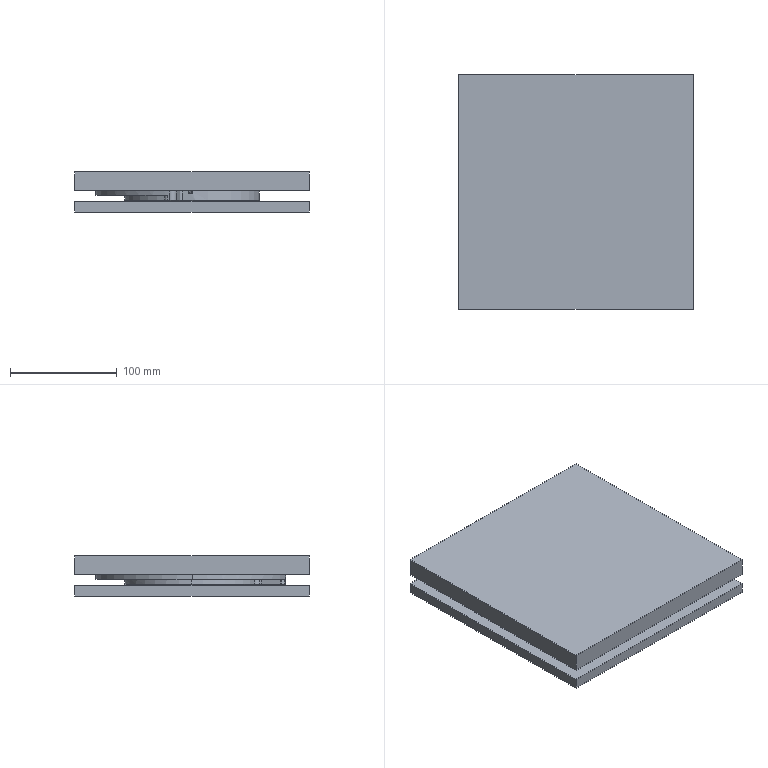NC program | NX | posted with a generic post | part box 220 x 220 x 37.5 mm
Lines 76 to 952 of 13716:
(ADAPTIVE_MILLING , TOOL : D10)
N120 T03 M6
N122 G54
N124 G17 G0 G90 X86.367 Y-45.277 S8000 M3
N126 G43 Z30. H3
N128 Z-14.
N130 G94 G1 Z-17. F1000.
N132 X84.574 Y-44.181 F3500.
N134 G3 X83.996 Y-44.309 R0.517
N136 X80.048 Y-49.358 R33.84
N138 G2 X66.319 Y-66.497 R105.778
N140 X-92.415 Y16.802 R93.928
N142 X-92.829 Y20.13 R11.157
N144 G3 X-93.451 Y20.622 R0.524
N146 G1 X-95.297 Y20.256
N148 G3 X-95.297 Y19.277 R0.523
N150 G1 Z-14.
N152 G0 Z30.
N154 X84.745 Y-47.205
N156 Z-14.
N158 G1 Z-17. F1000.
N160 G3 X85.138 Y-46.276 R0.505 F3500.
N162 G1 X83.355 Y-45.432
N164 G3 X82.875 Y-45.546 R0.516
N166 X78.753 Y-49.761 R17.096
N168 G2 X70.173 Y-60.818 R172.579
N170 X-91.735 Y14.531 R92.876
N172 G1 X-91.721 Y14.655
N174 X-91.709 Y14.779
N176 X-91.702 Y14.904
N178 X-91.718 Y15.028
N180 X-91.723 Y15.053
N182 G2 X-92.422 Y16.833 R12.053
N184 G3 X-93.208 Y17.162 R0.523
N186 G1 X-94.72 Y16.21
N188 G3 X-94.552 Y15.325 R0.523
N190 G1 Z-14.
N192 G0 Z30.
N194 X83.381 Y-48.311
N196 Z-14.
N198 G1 Z-17. F1000.
N200 G3 X83.835 Y-47.418 R0.505 F3500.
N202 G1 X82.268 Y-46.36
N204 G3 X81.746 Y-46.416 R0.514
N206 G2 X80.496 Y-47.163 R8.174
N208 G3 X77.305 Y-50.313 R15.899
N210 G2 X69.954 Y-59.478 R395.084
N212 X-90.974 Y12.49 R91.836
N214 G3 X-90.988 Y13.871 R3.68
N216 G2 X-91.754 Y15.127 R8.922
N218 G3 X-92.604 Y15.292 R0.523
N220 G1 X-93.829 Y14.054
N222 G3 X-93.578 Y13.261 R0.524
N224 G1 Z-14.
N226 G0 Z30.
N228 X82.131 Y-49.111
N230 Z-14.
N232 G1 Z-17. F1000.
N234 G3 X82.626 Y-48.25 R0.505 F3500.
N236 G1 X81.197 Y-47.049
N238 G3 X80.71 Y-47.033 R0.516
N240 X78.354 Y-48.358 R13.575
N242 X74.556 Y-52.323 R27.605
N244 G2 X65.409 Y-62.915 R164.628
N246 X-90.181 Y10.267 R90.765
N248 G3 X-90.157 Y12.759 R9.982
N250 X-90.653 Y13.361 R2.719
N252 G1 X-90.996 Y13.883
N254 G3 X-91.709 Y14.019 R0.507
N256 G1 X-93.073 Y13.05
N258 G3 X-92.887 Y12.216 R0.506
N260 G1 Z-14.
N262 G0 Z30.
N264 X80.927 Y-49.729
N266 Z-14.
N268 G1 Z-17. F1000.
N270 G3 X81.459 Y-48.902 R0.505 F3500.
N272 G1 X80.19 Y-47.603
N274 G3 X79.742 Y-47.523 R0.518
N276 X75.889 Y-49.733 R8.088
N278 X70.939 Y-55.194 R66.815
N280 G2 X58.211 Y-68.242 R108.748
N282 X-89.332 Y8.128 R89.703
N284 G3 X-89.304 Y11.744 R15.899
N286 G1 X-89.33 Y11.866
N288 X-89.376 Y11.983
N290 X-89.432 Y12.077
N292 X-90.295 Y12.98
N294 G3 X-90.994 Y13.011 R0.508
N296 G1 X-92.213 Y11.927
N298 G3 X-91.988 Y11.136 R0.507
N300 G1 Z-14.
N302 G0 Z30.
N304 X79.741 Y-50.13
N306 Z-14.
N308 G1 Z-17. F1000.
N310 G3 X80.32 Y-49.359 R0.505 F3500.
N312 G1 X79.288 Y-47.939
N314 G3 X78.784 Y-47.81 R0.514
N316 X76.695 Y-48.509 R11.339
N318 X72.855 Y-51.682 R16.957
N320 X65.561 Y-59.747 R993.743
N322 G2 X9.214 Y-88.161 R89.35
N324 X-88.406 Y6.532 R88.653
N326 G3 X-88.422 Y10.773 R20.785
N328 X-88.714 Y11.536 R1.595
N330 G1 X-89.35 Y11.998
N332 X-89.389 Y12.031
N334 X-89.475 Y12.122
N336 G3 X-90.244 Y12.076 R0.507
N338 G1 X-91.21 Y10.779
N340 G3 X-90.931 Y10.072 R0.507
N342 G1 Z-14.
N344 G0 Z30.
N346 X78.751 Y-50.429
N348 Z-14.
N350 G1 Z-17. F1000.
N352 G3 X79.348 Y-49.685 R0.505 F3500.
N354 G1 X78.418 Y-48.214
N356 G3 X77.983 Y-48.045 R0.517
N358 X74.203 Y-49.513 R6.431
N360 X69.408 Y-54.07 R36.849
N362 G2 X59.034 Y-64.722 R153.931
N364 X-87.451 Y5.032 R87.61
N366 G3 X-87.519 Y9.898 R25.802
N368 X-87.906 Y10.951 R2.017
N370 G1 X-88.715 Y11.537
N372 G3 X-89.438 Y11.399 R0.507
N374 G1 X-90.286 Y10.052
N376 G3 X-89.992 Y9.378 R0.507
N378 G1 Z-14.
N380 G0 Z30.
N382 X77.512 Y-50.61
N384 Z-14.
N386 G1 Z-17. F1000.
N388 G3 X78.146 Y-49.934 R0.506 F3500.
N390 G1 X77.47 Y-48.386
N392 G3 X76.989 Y-48.155 R0.513
N394 X72.903 Y-49.694 R7.007
N396 X67.694 Y-54.54 R40.76
N398 G2 X57.321 Y-64.841 R147.601
N400 X-86.479 Y2.946 R86.546
N402 G3 X-86.557 Y8.814 R40.487
N404 X-87.061 Y10.476 R4.512
N406 X-87.906 Y10.951 R3.058
N408 X-88.509 Y10.885 R0.51
N410 G1 X-89.688 Y9.772
N412 G3 X-89.456 Y8.992 R0.507
N414 G1 Z-14.
N416 G0 Z30.
N418 X76.508 Y-50.724
N420 Z-14.
N422 G1 Z-17. F1000.
N424 G3 X77.155 Y-50.078 R0.506 F3500.
N426 G1 X76.584 Y-48.502
N428 G3 X76.178 Y-48.244 R0.516
N430 X72.949 Y-48.977 R5.032
N432 X68.167 Y-52.774 R23.029
N434 G2 X60.321 Y-60.66 R868.911
N436 X17.03 Y-83.76 R86.865
N438 X-85.46 Y1.604 R85.487
N440 G3 X-85.609 Y7.973 R49.447
N442 X-86.267 Y10.105 R5.323
N444 X-87.303 Y10.657 R4.211
N446 X-87.985 Y10.401 R0.507
N448 G1 X-88.599 Y8.951
N450 G3 X-88.28 Y8.355 R0.508
N452 G1 Z-14.
N454 G0 Z30.
N456 X75.748 Y-50.717
N458 Z-14.
N460 G1 Z-17. F1000.
N462 G3 X76.408 Y-50.115 R0.506 F3500.
N464 G1 X75.982 Y-48.502
N466 G3 X75.555 Y-48.2 R0.514
N468 X71.611 Y-49.072 R5.827
N470 X66.358 Y-53.283 R27.528
N472 G2 X57.105 Y-62.233 R285.389
N474 X-22.068 Y-81.479 R84.739
N476 X-84.42 Y1.361 R84.539
N478 G3 X-84.713 Y7.598 R42.846
N480 X-85.578 Y9.91 R4.764
N482 X-86.252 Y10.155 R2.421
N484 G1 X-86.478 Y10.262
N486 G3 X-87.096 Y10.115 R0.509
N488 G1 X-88.072 Y8.837
N490 G3 X-87.797 Y8.126 R0.507
N492 G1 Z-14.
N494 G0 Z30.
N496 X74.669 Y-50.642
N498 Z-14.
N500 G1 Z-17. F1000.
N502 G3 X75.342 Y-50.103 R0.506 F3500.
N504 G1 X75.129 Y-48.493
N506 G3 X74.682 Y-48.138 R0.512
N508 X73.338 Y-48.022 R8.372
N510 X69.453 Y-49.64 R8.896
N512 X64.035 Y-54.253 R41.121
N514 G2 X53.368 Y-64.067 R172.763
N516 X-83.361 Y-0.32 R83.394
N518 G3 X-83.693 Y6.543 R61.748
N520 X-84.718 Y9.593 R6.709
N522 G1 X-84.801 Y9.686
N524 X-84.902 Y9.76
N526 X-84.99 Y9.807
N528 X-85.834 Y10.036
N530 G3 X-86.45 Y9.694 R0.508
N532 G1 X-86.896 Y8.181
N534 G3 X-86.567 Y7.645 R0.509
N536 G1 Z-14.
N538 G0 Z30.
N540 X74.105 Y-50.594
N542 Z-14.
N544 G1 Z-17. F1000.
N546 G3 X74.778 Y-50.056 R0.506 F3500.
N548 G1 X74.564 Y-48.419
N550 G3 X74.207 Y-48.077 R0.515
N552 X70.675 Y-48.288 R4.771
N554 X65.767 Y-51.471 R18.618
N556 X58.324 Y-58.334 R265.551
N558 G2 X38.9 Y-72.524 R91.967
N560 X-82.285 Y-1.651 R82.313
N562 G3 X-82.729 Y5.957 R72.331
N564 X-83.817 Y9.254 R8.109
N566 X-84.47 Y9.666 R0.828
N568 G1 X-85.073 Y9.83
N570 G3 X-85.699 Y9.449 R0.507
N572 G1 X-86.026 Y7.91
N574 G3 X-85.694 Y7.409 R0.51
N576 G1 Z-14.
N578 G0 Z30.
N580 X73.24 Y-50.406
N582 Z-14.
N584 G1 Z-17. F1000.
N586 G3 X73.918 Y-49.912 R0.507 F3500.
N588 G1 X73.851 Y-48.28
N590 G3 X73.481 Y-47.89 R0.514
N592 X69.671 Y-48.101 R5.133
N594 X64.343 Y-51.553 R20.596
N596 X56.082 Y-59.004 R405.756
N598 G2 X36.408 Y-72.62 R89.446
N600 X-81.179 Y-3.094 R81.248
N602 G3 X-81.711 Y5.135 R96.899
N604 X-82.901 Y8.924 R9.743
N606 X-83.488 Y9.492 R1.449
N608 G1 X-84.35 Y9.644
N610 G3 X-84.935 Y9.237 R0.507
N612 G1 X-85.21 Y7.685
N614 G3 X-84.878 Y7.198 R0.51
N616 G1 Z-14.
N618 G0 Z30.
N620 X72.201 Y-50.141
N622 Z-14.
N624 G1 Z-17. F1000.
N626 G3 X72.879 Y-49.685 R0.507 F3500.
N628 G1 X72.932 Y-48.078
N630 G3 X72.6 Y-47.663 R0.513
N632 X69.866 Y-47.501 R3.861
N634 X64.896 Y-50.062 R14.817
N636 X58.048 Y-55.894 R92.054
N638 G2 X45.619 Y-65.951 R118.839
N640 X-80.105 Y-3.568 R80.212
N642 G3 X-80.756 Y4.778 R92.475
N644 X-82.088 Y8.78 R10.206
N646 X-82.682 Y9.35 R1.491
N648 G1 X-83.544 Y9.502
N650 G3 X-84.133 Y9.066 R0.507
N652 G1 X-84.318 Y7.492
N654 G3 X-83.987 Y7.041 R0.512
N656 G1 Z-14.
N658 G0 Z30.
N660 X71.367 Y-49.848
N662 Z-14.
N664 G1 Z-17. F1000.
N666 G3 X72.007 Y-49.568 R0.508 F3500.
N668 G1 X72.606 Y-48.112
N670 G3 X72.326 Y-47.541 R0.509
N672 X68.936 Y-47.222 R4.324
N674 X63.74 Y-49.891 R15.977
N676 X56.554 Y-55.906 R102.667
N678 G2 X43.355 Y-66.192 R112.499
N680 X-79.021 Y-4.133 R79.167
N682 G3 X-79.796 Y4.454 R91.307
N684 X-81.27 Y8.67 R10.869
N686 X-81.843 Y9.202 R1.569
N688 G1 X-82.705 Y9.354
N690 G3 X-83.26 Y9.051 R0.512
N692 G1 X-83.881 Y7.562
N694 G3 X-83.563 Y6.966 R0.511
N696 G1 Z-14.
N698 G0 Z30.
N700 X71.078 Y-49.715
N702 Z-14.
N704 G1 Z-17. F1000.
N706 G3 X71.76 Y-49.294 R0.512 F3500.
N708 G1 X71.941 Y-47.668
N710 G3 X71.645 Y-47.226 R0.519
N712 X68.131 Y-46.887 R4.547
N714 X62.793 Y-49.552 R16.49
N716 X55.348 Y-55.646 R104.608
N718 G2 X40.868 Y-66.511 R108.174
N720 X-77.901 Y-5.089 R78.108
N722 G3 X-78.721 Y3.494 R117.25
N724 X-80.218 Y8.233 R13.248
N726 X-80.991 Y9.051 R1.926
N728 G1 X-81.852 Y9.203
N730 G3 X-82.413 Y8.883 R0.51
N732 G1 X-82.97 Y7.381
N734 G3 X-82.649 Y6.805 R0.509
N736 G1 Z-14.
N738 G0 Z30.
N740 X70.294 Y-49.355
N742 Z-14.
N744 G1 Z-17. F1000.
N746 G3 X70.966 Y-48.973 R0.509 F3500.
N748 G1 X71.258 Y-47.382
N750 G3 X70.964 Y-46.912 R0.514
N752 X67.886 Y-46.418 R4.123
N754 X62.533 Y-48.742 R14.766
N756 X55.061 Y-54.599 R79.752
N758 G2 X41.84 Y-64.655 R119.816
N760 X-76.751 Y-6.254 R77.047
N762 G3 X-77.721 Y3.068 R142.072
N764 X-79.247 Y7.933 R14.664
N766 X-80.113 Y8.897 R2.203
N768 G1 X-81.098 Y9.07
N770 G3 X-81.665 Y8.732 R0.509
N772 G1 X-82.161 Y7.211
N774 G3 X-81.836 Y6.662 R0.509
N776 G1 Z-14.
N778 G0 Z30.
N780 X69.384 Y-48.891
N782 Z-14.
N784 G1 Z-17. F1000.
N786 G3 X69.992 Y-48.674 R0.509 F3500.
N788 G1 X70.791 Y-47.316
N790 G3 X70.574 Y-46.693 R0.509
N792 X67.112 Y-46.033 R4.424
N794 X61.52 Y-48.429 R15.36
N796 X54.186 Y-54.057 R77.463
N798 G2 X41.309 Y-63.743 R126.175
N800 X-75.59 Y-7.267 R75.998
N802 G3 X-76.698 Y2.544 R174.092
N804 X-78.341 Y7.762 R15.754
N806 X-79.22 Y8.739 R2.223
N808 G1 X-80.205 Y8.913
N810 G3 X-80.775 Y8.565 R0.509
N812 G1 X-81.24 Y7.039
N814 G3 X-80.914 Y6.499 R0.509
N816 G1 Z-14.
N818 G0 Z30.
N820 X69.11 Y-48.733
N822 Z-14.
N824 G1 Z-17. F1000.
N826 G3 X69.78 Y-48.381 R0.512 F3500.
N828 G1 X70.177 Y-46.804
N830 G3 X69.924 Y-46.318 R0.518
N832 X66.343 Y-45.629 R4.585
N834 X60.618 Y-48.031 R15.844
N836 X53.809 Y-53.111 R72.764
N838 G2 X41.843 Y-62.143 R146.46
N840 X-32.178 Y-67.574 R75.192
N842 X-74.499 Y-7.548 R75.061
N844 G3 X-75.726 Y2.374 R170.304
N846 X-77.416 Y7.58 R16.3
N848 X-78.323 Y8.581 R2.263
N850 G1 X-79.308 Y8.755
N852 G3 X-79.88 Y8.4 R0.509
N854 G1 X-80.324 Y6.872
N856 G3 X-79.997 Y6.338 R0.509
N858 G1 Z-14.
N860 G0 Z30.
N862 X68.393 Y-48.319
N864 Z-14.
N866 G1 Z-17. F1000.
N868 G3 X69.052 Y-47.993 R0.509 F3500.
N870 G1 X69.524 Y-46.448
N872 G3 X69.275 Y-45.943 R0.514
N874 X65.578 Y-45.213 R4.742
N876 X59.932 Y-47.49 R15.988
N878 X53.059 Y-52.481 R68.743
N880 G2 X41.129 Y-61.355 R153.462
N882 X-20.52 Y-70.866 R74.359
N884 X-73.248 Y-9.08 R73.915
N886 G3 X-74.571 Y1.21 R390.61
N888 X-76.24 Y6.95 R20.325
N890 X-77.265 Y8.352 R4.627
N892 X-78.391 Y8.593 R5.382
N894 X-78.964 Y8.236 R0.508
N896 G1 X-79.398 Y6.706
N898 G3 X-79.07 Y6.174 R0.509
N900 G1 Z-14.
N902 G0 Z30.
N904 X67.578 Y-47.849
N906 Z-14.
N908 G1 Z-17. F1000.
N910 G3 X68.229 Y-47.545 R0.507 F3500.
N912 G1 X68.761 Y-46.037
N914 G3 X68.517 Y-45.505 R0.51
N916 X64.939 Y-44.767 R4.751
N918 X59.146 Y-47.003 R15.989
N920 X51.231 Y-52.685 R75.994
N922 G2 X38.947 Y-61.495 R138.42
N924 X-26.793 Y-67.595 R73.2
N926 X-72.139 Y-9.381 R72.911
N928 G3 X-73.555 Y0.896 R384.559
N930 X-75.348 Y6.859 R20.943
N932 X-76.411 Y8.226 R3.68
N934 G1 X-76.485 Y8.257
N936 X-77.47 Y8.431
N938 G3 X-78.043 Y8.073 R0.508
N940 G1 X-78.477 Y6.543
N942 G3 X-78.15 Y6.012 R0.509
N944 G1 Z-14.
N946 G0 Z30.
N948 X66.767 Y-47.381
N950 Z-14.
N952 G1 Z-17. F1000.
N954 G3 X67.41 Y-47.095 R0.508 F3500.
N956 G1 X67.999 Y-45.617
N958 G3 X67.759 Y-45.068 R0.51
N960 X64.053 Y-44.348 R4.931
N962 X57.928 Y-46.76 R17.069
N964 X49.689 Y-52.636 R89.664
N966 G2 X37.389 Y-61.206 R128.95
N968 X-32.584 Y-63.804 R72.032
N970 X-71.044 Y-9.564 R71.967
N972 G3 X-72.606 Y0.944 R299.425
N974 X-74.444 Y6.763 R20.566
N976 X-75.43 Y8.038 R4.3
N978 X-76.539 Y8.266 R11.317
N980 X-77.111 Y7.909 R0.508
N982 G1 X-77.545 Y6.379
N984 G3 X-77.218 Y5.848 R0.509
N986 G1 Z-14.
N988 G0 Z30.
N990 X66.101 Y-46.996
N992 Z-14.
N994 G1 Z-17. F1000.
N996 G3 X66.742 Y-46.717 R0.508 F3500.
N998 G1 X67.348 Y-45.248
N1000 G3 X67.11 Y-44.693 R0.51
N1002 X63.294 Y-43.9 R5.074
N1004 X57.144 Y-46.251 R17.239
N1006 X49.445 Y-51.59 R84.212
N1008 G2 X37.556 Y-59.88 R144.347
N1010 X-11.773 Y-69.586 R71.533
N1012 X-69.773 Y-10.869 R70.78
N1014 G3 X-71.458 Y0.001 R801.947
N1016 X-73.295 Y6.215 R24.669
N1018 X-74.436 Y7.842 R5.577
N1020 X-75.586 Y8.098 R4.111
N1022 X-76.161 Y7.732 R0.508
N1024 G1 X-76.566 Y6.198
N1026 G3 X-76.238 Y5.675 R0.51
N1028 G1 Z-14.
N1030 G0 Z30.
N1032 X65.325 Y-46.548
N1034 Z-14.
N1036 G1 Z-17. F1000.
N1038 G3 X65.963 Y-46.275 R0.508 F3500.
N1040 G1 X66.589 Y-44.816
N1042 G3 X66.352 Y-44.255 R0.51
N1044 X62.538 Y-43.443 R5.132
N1046 X56.365 Y-45.736 R17.413
N1048 X48.11 Y-51.368 R85.254
N1050 G2 X36.226 Y-59.443 R137.297
N1052 X-19.674 Y-66.662 R70.27
N1054 X-68.706 Y-10.821 R69.795
N1056 G3 X-70.542 Y0.278 R462.541
N1058 X-72.487 Y6.326 R22.468
N1060 X-73.542 Y7.705 R4.592
N1062 X-74.65 Y7.933 R11.921
N1064 X-75.236 Y7.513 R0.507
N1066 G1 X-75.472 Y5.946
N1068 G3 X-75.142 Y5.481 R0.512
N1070 G1 Z-14.
N1072 G0 Z30.
N1074 X64.56 Y-46.107
N1076 Z-14.
N1078 G1 Z-17. F1000.
N1080 G3 X65.198 Y-45.836 R0.508 F3500.
N1082 G1 X65.831 Y-44.381
N1084 G3 X65.594 Y-43.818 R0.51
N1086 X61.659 Y-42.996 R5.246
N1088 X55.587 Y-45.21 R17.735
N1090 X47.176 Y-50.835 R86.711
N1092 G2 X34.897 Y-58.993 R133.657
N1094 X-18.089 Y-66. R69.271
N1096 X-67.485 Y-11.64 R68.736
N1098 G3 X-69.423 Y-0.432 R902.29
N1100 X-71.436 Y5.989 R25.143
N1102 X-72.638 Y7.562 R4.16
N1104 G1 X-72.707 Y7.591
N1106 X-73.691 Y7.764
N1108 G3 X-74.276 Y7.358 R0.507
N1110 G1 X-74.552 Y5.806
N1112 G3 X-74.223 Y5.319 R0.51
N1114 G1 Z-14.
N1116 G0 Z30.
N1118 X63.803 Y-45.669
N1120 Z-14.
N1122 G1 Z-17. F1000.
N1124 G3 X64.44 Y-45.399 R0.508 F3500.
N1126 G1 X65.073 Y-43.943
N1128 G3 X64.836 Y-43.38 R0.51
N1130 X60.906 Y-42.526 R5.297
N1132 X54.485 Y-44.862 R18.154
N1134 X45.736 Y-50.658 R95.431
N1136 X42.203 Y-53.51 R36.5
N1138 G1 X38.136 Y-56.48
N1140 X38.119 Y-56.492
N1142 X33.843 Y-59.152
N1144 X33.825 Y-59.163
N1146 X29.364 Y-61.499
N1148 X29.345 Y-61.508
N1150 X24.724 Y-63.507
N1152 X24.704 Y-63.514
N1154 X19.947 Y-65.165
N1156 X19.927 Y-65.171
N1158 X15.06 Y-66.465
N1160 X15.04 Y-66.469
N1162 X10.091 Y-67.398
N1164 X10.07 Y-67.402
N1166 X5.065 Y-67.961
N1168 X5.045 Y-67.963
N1170 X0.002 Y-68.15
N1172 X-5.134 Y-67.956
N1174 X-5.155 Y-67.954
N1176 X-10.251 Y-67.374
N1178 X-10.272 Y-67.371
N1180 X-15.31 Y-66.408
N1182 X-15.33 Y-66.403
N1184 X-20.281 Y-65.062
N1186 X-20.301 Y-65.056
N1188 X-25.136 Y-63.345
N1190 X-25.156 Y-63.337
N1192 X-29.848 Y-61.265
N1194 X-29.867 Y-61.256
N1196 X-34.39 Y-58.836
N1198 X-34.408 Y-58.826
N1200 X-38.735 Y-56.071
N1202 X-38.752 Y-56.059
N1204 X-42.858 Y-52.986
N1206 X-42.875 Y-52.973
N1208 X-46.737 Y-49.598
N1210 X-46.753 Y-49.584
N1212 X-50.35 Y-45.927
N1214 X-50.364 Y-45.911
N1216 X-53.674 Y-41.994
N1218 X-53.687 Y-41.977
N1220 X-56.692 Y-37.82
N1222 X-56.704 Y-37.803
N1224 X-59.386 Y-33.431
N1226 X-59.397 Y-33.413
N1228 X-61.741 Y-28.851
N1230 X-61.75 Y-28.832
N1232 X-63.744 Y-24.106
N1234 X-63.751 Y-24.086
N1236 X-65.382 Y-19.223
N1238 X-65.388 Y-19.203
N1240 X-66.647 Y-14.231
N1242 X-66.652 Y-14.21
N1244 X-67.532 Y-9.157
N1246 X-67.534 Y-9.136
N1248 G3 X-68.392 Y-1.159 R141.378
N1250 X-70.446 Y5.767 R24.619
N1252 X-71.622 Y7.365 R5.084
N1254 X-72.734 Y7.595 R8.834
N1256 X-73.363 Y6.923 R0.551
N1258 G1 X-72.651 Y5.054 Z-16.9
N1260 X-70.616 Y-0.252
N1262 X-69.9 Y-2.119 Z-17.
N1264 X-69.056 Y-4.3
N1266 G3 X-68.032 Y-4.01 R0.55
N1268 X-68.201 Y1.11 R67.977
N1270 X-70.205 Y6.706 R12.59
N1272 X-70.809 Y7.256 R1.69
N1274 G1 X-71.794 Y7.43
N1276 G3 X-72.384 Y6.649 R0.551
N1278 G1 X-69.123 Y-0.088
N1280 G3 X-68.122 Y0.239 R0.55
N1282 G2 X-68.09 Y2.759 R104.092
N1284 G3 X-69.652 Y6.901 R7.194
N1286 G1 X-69.741 Y6.989
N1288 X-69.846 Y7.058
N1290 X-69.961 Y7.107
N1292 X-70.823 Y7.259
N1294 G3 X-71.407 Y6.464 R0.551
N1296 G1 X-69.069 Y1.961
N1298 G3 X-68.079 Y2.259 R0.551
N1300 X-68.086 Y4.876 R10.598
N1302 X-69.052 Y6.873 R3.968
N1304 X-70.001 Y7.114 R2.516
N1306 X-70.571 Y6.294 R0.551
N1308 G1 X-68.964 Y3.562
N1310 G3 X-67.991 Y3.882 R0.551
N1312 X-68.08 Y5.989 R5.552
N1314 X-68.751 Y6.893 R1.35
N1316 G1 X-69.366 Y7.002
N1318 G3 X-69.914 Y6.148 R0.551
N1320 G1 X-68.874 Y4.653
N1322 G3 X-67.93 Y5.005 R0.551
N1324 X-68.051 Y6.48 R2.883
N1326 X-68.816 Y6.905 R0.857
N1328 X-69.337 Y6.015 R0.551
N1330 G1 X-68.803 Y5.373
N1332 G3 X-67.889 Y5.754 R0.551
N1334 X-67.994 Y6.595 R1.279
N1336 X-68.499 Y6.849 R0.878
N1338 X-68.91 Y6.772 R0.63
N1340 G1 X-70.702 Y5.686
N1342 G3 X-70.531 Y4.669 R0.597
N1344 G1 Z-14.
N1346 G0 Z30.
N1348 X63.045 Y-45.232
N1350 Z-14.
N1352 G1 Z-17. F1000.
N1354 G3 X63.684 Y-44.961 R0.508 F3500.
N1356 G1 X64.315 Y-43.505
N1358 G3 X64.079 Y-42.943 R0.51
N1360 X60.03 Y-42.063 R5.422
N1362 X53.709 Y-44.321 R18.66
N1364 X49.349 Y-46.979 R71.69
N1366 G1 X46.069 Y-50.219
N1368 X46.054 Y-50.234
N1370 X44.626 Y-51.449
N1372 G3 X45.228 Y-52.36 R0.55
N1374 G1 X47.922 Y-51.017
N1376 X49.712 Y-50.125 Z-16.9
N1378 X61.396 Y-44.302
N1380 X63.186 Y-43.409 Z-17.
N1382 G3 X63.213 Y-42.443 R0.551
N1384 X59.28 Y-41.584 R5.413
N1386 X53.047 Y-43.719 R18.361
N1388 G1 X52.825 Y-43.836
N1390 X52.605 Y-43.954
N1392 X52.166 Y-44.193
N1394 X51.839 Y-44.376
N1396 X51.621 Y-44.5
N1398 X51.514 Y-44.564
N1400 X51.472 Y-44.595
N1402 G2 X49.296 Y-47.032 R68.293
N1404 G3 X49.885 Y-47.935 R0.55
N1406 G1 X51.047 Y-47.475
N1408 X52.907 Y-46.74 Z-16.9
N1410 X60.456 Y-43.754
N1412 X62.316 Y-43.019 Z-17.
N1414 G3 X62.455 Y-42.005 R0.554
N1416 X58.406 Y-41.112 R5.513
N1418 X52.993 Y-42.85 R16.487
N1420 G1 X52.976 Y-42.871
N1422 X51.415 Y-44.66
N1424 G3 X51.997 Y-45.546 R0.55
N1426 G1 X61.565 Y-42.47
N1428 G3 X61.589 Y-41.505 R0.551
N1430 X57.658 Y-40.619 R5.484
N1432 X53.935 Y-41.613 R11.166
N1434 G1 X53.892 Y-41.65
N1436 X52.989 Y-42.854
N1438 G3 X53.553 Y-43.72 R0.551
N1440 G1 X60.763 Y-42.053
N1442 G3 X60.831 Y-41.068 R0.551
N1444 X56.788 Y-40.136 R5.589
N1446 X54.725 Y-40.607 R7.529
N1448 X53.852 Y-41.703 R6.836
N1450 X54.392 Y-42.574 R0.551
N1452 G1 X59.875 Y-41.562
N1454 G3 X59.965 Y-40.568 R0.551
N1456 X55.319 Y-39.85 R5.283
N1458 X54.548 Y-40.774 R3.656
N1460 X55.068 Y-41.648 R0.551
N1462 G1 X58.992 Y-41.068
N1464 G3 X59.099 Y-40.068 R0.551
N1466 X56.291 Y-39.198 R4.57
N1468 X55.547 Y-39.442 R1.289
N1470 G1 X55.097 Y-40.042
N1472 G3 X55.611 Y-40.917 R0.551
N1474 G1 X58.121 Y-40.569
N1476 G3 X58.233 Y-39.568 R0.551
N1478 X56.389 Y-38.884 R3.466
N1480 X55.807 Y-39.094 R0.897
N1482 G1 X55.507 Y-39.494
N1484 G3 X56.042 Y-40.366 R0.551
N1486 G1 X57.381 Y-40.126
N1488 G3 X57.475 Y-39.13 R0.551
N1490 X56.324 Y-38.707 R2.025
N1492 X55.733 Y-39.193 R0.951
N1494 X56.322 Y-40.052 R0.55
N1496 G1 X56.996 Y-39.857
N1498 G3 X57.042 Y-38.88 R0.551
N1500 X56.094 Y-38.763 R0.805
N1502 G1 X55.958 Y-38.893
N1504 G3 X55.893 Y-39.51 R0.615
N1506 G1 X56.933 Y-41.761
N1508 Z-14.
N1510 G0 Z30.
N1512 X41.169 Y-27.555
N1514 Z3.
N1516 G3 X41.169 Y-27.555 Z2.506 I0.978 J4.392 F1000.
N1518 X41.169 Y-27.555 Z2.013 I0.978 J4.392
N1520 X41.169 Y-27.555 Z1.519 I0.978 J4.392
N1522 X41.169 Y-27.555 Z1.026 I0.978 J4.392
N1524 X41.169 Y-27.555 Z0.532 I0.978 J4.392
N1526 X41.169 Y-27.555 Z0.039 I0.978 J4.392
N1528 X41.169 Y-27.555 Z-0.455 I0.978 J4.392
N1530 X41.169 Y-27.555 Z-0.948 I0.978 J4.392
N1532 X41.169 Y-27.555 Z-1.442 I0.978 J4.392
N1534 X41.169 Y-27.555 Z-1.935 I0.978 J4.392
N1536 X41.169 Y-27.555 Z-2.429 I0.978 J4.392
N1538 X41.169 Y-27.555 Z-2.922 I0.978 J4.392
N1540 X41.169 Y-27.555 Z-3.416 I0.978 J4.392
N1542 X41.169 Y-27.555 Z-3.909 I0.978 J4.392
N1544 X41.169 Y-27.555 Z-4.403 I0.978 J4.392
N1546 X41.169 Y-27.555 Z-4.896 I0.978 J4.392
N1548 X41.169 Y-27.555 Z-5.39 I0.978 J4.392
N1550 X41.169 Y-27.555 Z-5.884 I0.978 J4.392
N1552 X41.169 Y-27.555 Z-6.377 I0.978 J4.392
N1554 X41.169 Y-27.555 Z-6.871 I0.978 J4.392
N1556 X41.169 Y-27.555 Z-7.364 I0.978 J4.392
N1558 X41.169 Y-27.555 Z-7.858 I0.978 J4.392
N1560 X41.169 Y-27.555 Z-8.351 I0.978 J4.392
N1562 X41.169 Y-27.555 Z-8.845 I0.978 J4.392
N1564 X41.169 Y-27.555 Z-9.338 I0.978 J4.392
N1566 X41.169 Y-27.555 Z-9.832 I0.978 J4.392
N1568 X42.148 Y-27.663 Z-9.849 R4.5
N1570 X39.542 Y-26.842 R-4.501 F3500.
N1572 X47.015 Y-22.173 R4.667
N1574 X38.677 Y-26.748 R-4.976
N1576 X47.243 Y-21.2 R5.196
N1578 X38.066 Y-26.845 R-5.476
N1580 X47.622 Y-20.755 R5.721
N1582 X37.266 Y-26.686 R-5.998
N1584 X48.12 Y-20.555 R6.258
N1586 X36.698 Y-26.82 R-6.538
N1588 X48.608 Y-20.278 R6.812
N1590 X35.956 Y-26.695 R-7.101
N1592 X39.559 Y-29.925 R7.366
N1594 X47.26 Y-28.725 R7.205
N1596 X49.446 Y-24.684 R27.688
N1598 X47.457 Y-17.596 R6.995
N1600 X43.87 Y-15.675 R7.432
N1602 G2 X41.937 Y-15.892 R26.771
N1604 G3 X37.183 Y-17.312 R5.823
N1606 X35.92 Y-19.03 R3.431
N1608 X34.594 Y-22.002 R8.561
N1610 X41.968 Y-31.151 R7.898
N1612 X46.4 Y-30.1 R7.787
N1614 X47.265 Y-28.716 R14.67
N1616 G1 X49.262 Y-25.149
N1618 G3 X50.125 Y-22.95 R7.323
N1620 X47.566 Y-16.854 R7.119
N1622 X44.862 Y-15.351 R6.459
N1624 X43.645 Y-15.721 R6.52
N1626 X43.31 Y-16.445 R0.552
N1628 G1 X43.534 Y-16.791 Z-9.828
N1630 X43.781 Y-17.121 Z-9.808
N1632 X44.473 Y-18.071 Z-9.749
N1634 X47.74 Y-22.553
N1636 X48.922 Y-24.166 Z-9.849
N1638 G3 X49.812 Y-24.027 R0.551
N1640 X50.549 Y-21.545 R4.888
N1642 X47.344 Y-15.865 R7.424
N1644 X45.55 Y-15.041 R3.797
N1646 G1 X45.427 Y-15.065
N1648 X45.342 Y-15.095
N1650 X45.186 Y-15.192
N1652 X45.127 Y-15.22
N1654 X44.654 Y-15.38
N1656 G3 X44.381 Y-16.218 R0.551
N1658 G1 X49.365 Y-23.271
N1660 G3 X50.253 Y-23.129 R0.551
N1662 X50.562 Y-19.099 R4.444
N1664 X46.74 Y-14.848 R7.214
N1666 X45.866 Y-14.768 R1.279
N1668 G1 X45.336 Y-15.099
N1670 G3 X45.179 Y-15.885 R0.552
N1672 G1 X49.811 Y-22.352
N1674 G3 X50.712 Y-22.164 R0.551
N1676 X50.654 Y-17.95 R4.618
N1678 X47.334 Y-14.529 R6.644
N1680 X46.405 Y-14.432 R1.367
N1682 G1 X45.769 Y-14.829
N1684 G3 X45.622 Y-15.629 R0.552
N1686 G1 X50.142 Y-21.549
N1688 G3 X51.031 Y-21.349 R0.551
N1690 X50.966 Y-17.376 R4.364
N1692 X47.789 Y-14.17 R6.051
N1694 X46.723 Y-14.171 R1.148
N1696 G1 X46.317 Y-14.487
N1698 G3 X46.171 Y-15.287 R0.552
N1700 G1 X50.415 Y-20.85
N1702 G3 X51.305 Y-20.651 R0.551
N1704 X51.255 Y-16.801 R4.182
N1706 X48.097 Y-13.773 R5.486
N1708 X46.718 Y-14.176 R1.109
N1710 X46.676 Y-14.904 R0.554
N1712 G1 X50.741 Y-20.041
N1714 G3 X51.624 Y-19.836 R0.551
N1716 X51.529 Y-16.226 R3.962
N1718 X48.38 Y-13.383 R5.084
N1720 X47.068 Y-13.824 R1.119
N1722 X47.029 Y-14.556 R0.554
N1724 G1 X50.972 Y-19.462
N1726 G3 X51.852 Y-19.254 R0.551
N1728 X51.721 Y-15.54 R3.868
N1730 X48.64 Y-12.997 R4.722
N1732 X47.696 Y-13.192 R0.961
N1734 G1 X47.344 Y-13.546
N1736 G3 X47.32 Y-14.297 R0.553
N1738 G1 X51.262 Y-18.779
N1740 G3 X52.126 Y-18.556 R0.551
N1742 X51.846 Y-14.797 R3.794
N1744 X48.806 Y-12.605 R4.335
N1746 X47.696 Y-13.192 R0.969
N1748 X47.73 Y-13.911 R0.554
N1750 G1 X51.58 Y-17.947
N1752 G3 X52.439 Y-17.666 R0.551
N1754 X51.881 Y-14.008 R3.698
N1756 X48.872 Y-12.223 R3.932
N1758 X47.875 Y-12.915 R1.024
N1760 X47.966 Y-13.602 R0.554
N1762 G1 X51.816 Y-17.243
N1764 G3 X52.654 Y-16.948 R0.551
N1766 X52.02 Y-13.432 R3.483
N1768 X49.042 Y-11.844 R3.768
N1770 X48.364 Y-12.12 R0.942
N1772 G1 X48.102 Y-12.546
N1774 G3 X48.203 Y-13.243 R0.554
N1776 G1 X52.006 Y-16.652
N1778 G3 X52.833 Y-16.349 R0.551
N1780 X52.131 Y-12.863 R3.327
N1782 X49.193 Y-11.467 R3.599
N1784 X48.566 Y-11.792 R0.821
N1786 G1 X48.304 Y-12.218
N1788 G3 X48.421 Y-12.929 R0.554
N1790 G1 X52.208 Y-16.067
N1792 G3 X53.013 Y-15.75 R0.552
N1794 X52.378 Y-12.49 R3.128
N1796 X49.323 Y-11.097 R3.516
N1798 X48.566 Y-11.792 R0.832
N1800 X48.714 Y-12.449 R0.555
N1802 G1 X52.389 Y-15.47
N1804 G3 X53.192 Y-15.151 R0.552
N1806 X52.525 Y-12.022 R2.994
N1808 X49.436 Y-10.727 R3.427
N1810 X48.672 Y-11.496 R0.884
N1812 X48.853 Y-12.102 R0.555
N1814 G1 X52.543 Y-14.996
N1816 G3 X53.335 Y-14.672 R0.552
N1818 X52.66 Y-11.554 R2.919
N1820 X49.537 Y-10.353 R3.383
N1822 X48.913 Y-10.77 R0.927
N1824 G1 X48.755 Y-11.245
N1826 G3 X48.958 Y-11.866 R0.555
N1828 G1 X52.707 Y-14.528
N1830 G3 X53.479 Y-14.193 R0.552
N1832 X52.733 Y-11.039 R2.868
N1834 X49.562 Y-9.998 R3.294
N1836 X49.041 Y-10.383 R0.885
N1838 G1 X48.884 Y-10.857
N1840 G3 X49.109 Y-11.494 R0.555
N1842 G1 X52.909 Y-13.916
N1844 G3 X53.666 Y-13.525 R0.552
N1846 X52.733 Y-10.48 R2.872
N1848 X49.625 Y-9.629 R3.212
N1850 X49.095 Y-10.221 R0.722
N1852 G1 X49.016 Y-10.459
N1854 G3 X49.248 Y-11.099 R0.554
N1856 G1 X53.019 Y-13.43
N1858 G3 X53.769 Y-13.036 R0.552
N1860 X52.808 Y-10.011 R2.792
N1862 X49.678 Y-9.262 R3.167
N1864 X49.116 Y-10.111 R0.866
N1866 X49.387 Y-10.678 R0.555